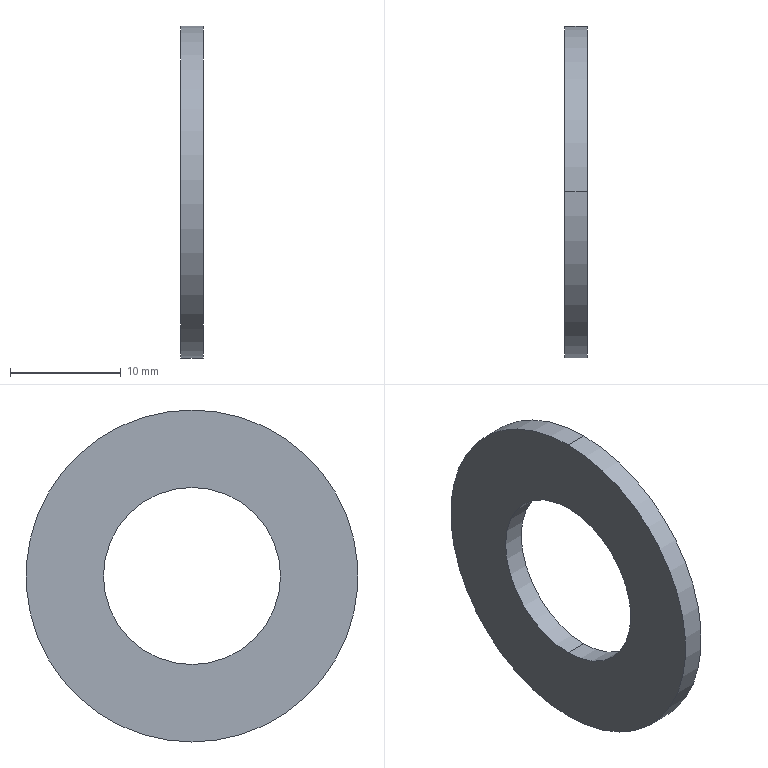Part | STEP file | WSJJ30-16-2 | 1 solid | 6 faces | box 2 x 30 x 30 mm | volume 1012 mm3 | cylinder 4 | plane 2 | commonest cylinder face diameters 16 x2 30 x2
STEP:
#1=CARTESIAN_POINT('',(2.,0.,-8.));
#2=VERTEX_POINT('',#1);
#3=CARTESIAN_POINT('',(2.,0.,8.));
#4=VERTEX_POINT('',#3);
#5=CARTESIAN_POINT('',(2.,0.,0.));
#6=DIRECTION('',(-1.,0.,0.));
#7=DIRECTION('',(0.,0.,1.));
#8=AXIS2_PLACEMENT_3D('',#5,#6,#7);
#9=CIRCLE('',#8,8.);
#10=EDGE_CURVE('',#2,#4,#9,.T.);
#11=ORIENTED_EDGE('',*,*,#10,.F.);
#12=CARTESIAN_POINT('',(0.,0.,-8.));
#13=VERTEX_POINT('',#12);
#14=CARTESIAN_POINT('',(0.,0.,-8.));
#15=DIRECTION('',(-1.,0.,0.));
#16=VECTOR('',#15,1000.);
#17=LINE('',#14,#16);
#18=EDGE_CURVE('',#2,#13,#17,.T.);
#19=ORIENTED_EDGE('',*,*,#18,.T.);
#20=CARTESIAN_POINT('',(0.,0.,8.));
#21=VERTEX_POINT('',#20);
#22=CARTESIAN_POINT('',(0.,0.,0.));
#23=DIRECTION('',(-1.,0.,0.));
#24=DIRECTION('',(0.,0.,1.));
#25=AXIS2_PLACEMENT_3D('',#22,#23,#24);
#26=CIRCLE('',#25,8.);
#27=EDGE_CURVE('',#13,#21,#26,.T.);
#28=ORIENTED_EDGE('',*,*,#27,.T.);
#29=CARTESIAN_POINT('',(0.,0.,8.));
#30=DIRECTION('',(-1.,0.,0.));
#31=VECTOR('',#30,1000.);
#32=LINE('',#29,#31);
#33=EDGE_CURVE('',#4,#21,#32,.T.);
#34=ORIENTED_EDGE('',*,*,#33,.F.);
#35=EDGE_LOOP('',(#11,#19,#28,#34));
#36=FACE_OUTER_BOUND('',#35,.T.);
#37=CARTESIAN_POINT('',(0.,0.,0.));
#38=DIRECTION('',(-1.,0.,0.));
#39=DIRECTION('',(0.,0.,1.));
#40=AXIS2_PLACEMENT_3D('',#37,#38,#39);
#41=CYLINDRICAL_SURFACE('',#40,8.);
#42=ADVANCED_FACE('',(#36),#41,.F.);
#43=CARTESIAN_POINT('',(2.,0.,15.));
#44=VERTEX_POINT('',#43);
#45=CARTESIAN_POINT('',(2.,0.,-15.));
#46=VERTEX_POINT('',#45);
#47=CARTESIAN_POINT('',(2.,0.,0.));
#48=DIRECTION('',(-1.,0.,0.));
#49=DIRECTION('',(0.,0.,1.));
#50=AXIS2_PLACEMENT_3D('',#47,#48,#49);
#51=CIRCLE('',#50,15.);
#52=EDGE_CURVE('',#44,#46,#51,.T.);
#53=ORIENTED_EDGE('',*,*,#52,.T.);
#54=CARTESIAN_POINT('',(0.,0.,-15.));
#55=VERTEX_POINT('',#54);
#56=CARTESIAN_POINT('',(0.,0.,-15.));
#57=DIRECTION('',(-1.,0.,0.));
#58=VECTOR('',#57,1000.);
#59=LINE('',#56,#58);
#60=EDGE_CURVE('',#46,#55,#59,.T.);
#61=ORIENTED_EDGE('',*,*,#60,.T.);
#62=CARTESIAN_POINT('',(0.,0.,15.));
#63=VERTEX_POINT('',#62);
#64=CARTESIAN_POINT('',(0.,0.,0.));
#65=DIRECTION('',(-1.,0.,0.));
#66=DIRECTION('',(0.,0.,1.));
#67=AXIS2_PLACEMENT_3D('',#64,#65,#66);
#68=CIRCLE('',#67,15.);
#69=EDGE_CURVE('',#63,#55,#68,.T.);
#70=ORIENTED_EDGE('',*,*,#69,.F.);
#71=CARTESIAN_POINT('',(0.,0.,15.));
#72=DIRECTION('',(-1.,0.,0.));
#73=VECTOR('',#72,1000.);
#74=LINE('',#71,#73);
#75=EDGE_CURVE('',#44,#63,#74,.T.);
#76=ORIENTED_EDGE('',*,*,#75,.F.);
#77=EDGE_LOOP('',(#53,#61,#70,#76));
#78=FACE_OUTER_BOUND('',#77,.T.);
#79=CARTESIAN_POINT('',(0.,0.,0.));
#80=DIRECTION('',(-1.,0.,0.));
#81=DIRECTION('',(0.,0.,1.));
#82=AXIS2_PLACEMENT_3D('',#79,#80,#81);
#83=CYLINDRICAL_SURFACE('',#82,15.);
#84=ADVANCED_FACE('',(#78),#83,.T.);
#85=CARTESIAN_POINT('',(0.,0.,0.));
#86=DIRECTION('',(-1.,0.,0.));
#87=DIRECTION('',(0.,0.,1.));
#88=AXIS2_PLACEMENT_3D('',#85,#86,#87);
#89=CIRCLE('',#88,8.);
#90=EDGE_CURVE('',#21,#13,#89,.T.);
#91=ORIENTED_EDGE('',*,*,#90,.F.);
#92=ORIENTED_EDGE('',*,*,#27,.F.);
#93=EDGE_LOOP('',(#91,#92));
#94=FACE_BOUND('',#93,.T.);
#95=ORIENTED_EDGE('',*,*,#69,.T.);
#96=CARTESIAN_POINT('',(0.,0.,0.));
#97=DIRECTION('',(-1.,0.,0.));
#98=DIRECTION('',(0.,0.,1.));
#99=AXIS2_PLACEMENT_3D('',#96,#97,#98);
#100=CIRCLE('',#99,15.);
#101=EDGE_CURVE('',#55,#63,#100,.T.);
#102=ORIENTED_EDGE('',*,*,#101,.T.);
#103=EDGE_LOOP('',(#95,#102));
#104=FACE_OUTER_BOUND('',#103,.T.);
#105=CARTESIAN_POINT('',(0.,8.,0.));
#106=DIRECTION('',(1.,0.,0.));
#107=DIRECTION('',(0.,0.,-1.));
#108=AXIS2_PLACEMENT_3D('',#105,#106,#107);
#109=PLANE('',#108);
#110=ADVANCED_FACE('',(#94,#104),#109,.F.);
#111=ORIENTED_EDGE('',*,*,#60,.F.);
#112=CARTESIAN_POINT('',(2.,0.,0.));
#113=DIRECTION('',(-1.,0.,0.));
#114=DIRECTION('',(0.,0.,1.));
#115=AXIS2_PLACEMENT_3D('',#112,#113,#114);
#116=CIRCLE('',#115,15.);
#117=EDGE_CURVE('',#46,#44,#116,.T.);
#118=ORIENTED_EDGE('',*,*,#117,.T.);
#119=ORIENTED_EDGE('',*,*,#75,.T.);
#120=ORIENTED_EDGE('',*,*,#101,.F.);
#121=EDGE_LOOP('',(#111,#118,#119,#120));
#122=FACE_OUTER_BOUND('',#121,.T.);
#123=CARTESIAN_POINT('',(0.,0.,0.));
#124=DIRECTION('',(-1.,0.,0.));
#125=DIRECTION('',(0.,0.,1.));
#126=AXIS2_PLACEMENT_3D('',#123,#124,#125);
#127=CYLINDRICAL_SURFACE('',#126,15.);
#128=ADVANCED_FACE('',(#122),#127,.T.);
#129=ORIENTED_EDGE('',*,*,#52,.F.);
#130=ORIENTED_EDGE('',*,*,#117,.F.);
#131=EDGE_LOOP('',(#129,#130));
#132=FACE_OUTER_BOUND('',#131,.T.);
#133=CARTESIAN_POINT('',(2.,0.,0.));
#134=DIRECTION('',(-1.,0.,0.));
#135=DIRECTION('',(0.,0.,1.));
#136=AXIS2_PLACEMENT_3D('',#133,#134,#135);
#137=CIRCLE('',#136,8.);
#138=EDGE_CURVE('',#4,#2,#137,.T.);
#139=ORIENTED_EDGE('',*,*,#138,.T.);
#140=ORIENTED_EDGE('',*,*,#10,.T.);
#141=EDGE_LOOP('',(#139,#140));
#142=FACE_BOUND('',#141,.T.);
#143=CARTESIAN_POINT('',(2.,8.,0.));
#144=DIRECTION('',(-1.,0.,0.));
#145=DIRECTION('',(0.,0.,1.));
#146=AXIS2_PLACEMENT_3D('',#143,#144,#145);
#147=PLANE('',#146);
#148=ADVANCED_FACE('',(#132,#142),#147,.F.);
#149=ORIENTED_EDGE('',*,*,#18,.F.);
#150=ORIENTED_EDGE('',*,*,#138,.F.);
#151=ORIENTED_EDGE('',*,*,#33,.T.);
#152=ORIENTED_EDGE('',*,*,#90,.T.);
#153=EDGE_LOOP('',(#149,#150,#151,#152));
#154=FACE_OUTER_BOUND('',#153,.T.);
#155=CARTESIAN_POINT('',(0.,0.,0.));
#156=DIRECTION('',(-1.,0.,0.));
#157=DIRECTION('',(0.,0.,1.));
#158=AXIS2_PLACEMENT_3D('',#155,#156,#157);
#159=CYLINDRICAL_SURFACE('',#158,8.);
#160=ADVANCED_FACE('',(#154),#159,.F.);
#161=CLOSED_SHELL('',(#42,#84,#110,#128,#148,#160));
#162=MANIFOLD_SOLID_BREP('',#161);
#163=CARTESIAN_POINT('',(0.,0.,0.));
#164=DIRECTION('',(0.,0.,1.));
#165=DIRECTION('',(1.,0.,0.));
#166=AXIS2_PLACEMENT_3D('',#163,#164,#165);
#167=(LENGTH_UNIT()NAMED_UNIT(*)SI_UNIT(.MILLI.,.METRE.));
#168=UNCERTAINTY_MEASURE_WITH_UNIT(LENGTH_MEASURE(0.00001),#167,'','');
#169=(NAMED_UNIT(*)PLANE_ANGLE_UNIT()SI_UNIT($,.RADIAN.));
#170=(NAMED_UNIT(*)SI_UNIT($,.STERADIAN.)SOLID_ANGLE_UNIT());
#171=(GEOMETRIC_REPRESENTATION_CONTEXT(3)GLOBAL_UNCERTAINTY_ASSIGNED_CONTEXT((#168))GLOBAL_UNIT_ASSIGNED_CONTEXT((#167,#169,#170))REPRESENTATION_CONTEXT('',''));
#172=ADVANCED_BREP_SHAPE_REPRESENTATION('',(#162,#166),#171);